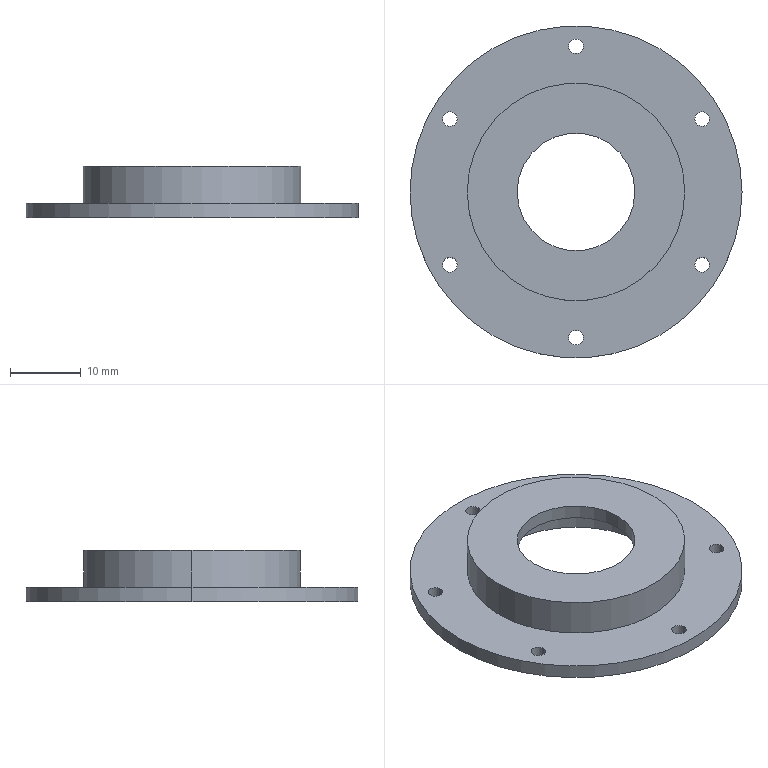Part | SolidWorks | features BaseBody 1 | 1 solid | 24 faces | box 47.022 x 47.022 x 7.237 mm | volume 3944 mm3 | cylinder 20 | plane 4 | commonest cylinder face diameters 2.063 x12 16.673 x2 26.799 x2 30.799 x2 47.022 x2
STEP:
#1=CARTESIAN_POINT('',(17.927,0.,0.));
#2=VERTEX_POINT('',#1);
#3=CARTESIAN_POINT('',(-8.872,0.,0.));
#4=VERTEX_POINT('',#3);
#5=CARTESIAN_POINT('',(4.528,0.,0.));
#6=DIRECTION('',(0.,0.,-1.));
#7=DIRECTION('',(1.,0.,0.));
#8=AXIS2_PLACEMENT_3D('',#5,#6,#7);
#9=CIRCLE('',#8,13.4);
#10=EDGE_CURVE('',#2,#4,#9,.T.);
#11=ORIENTED_EDGE('',*,*,#10,.T.);
#12=CARTESIAN_POINT('',(-8.872,0.,5.237));
#13=VERTEX_POINT('',#12);
#14=CARTESIAN_POINT('',(-8.872,0.,0.));
#15=DIRECTION('',(0.,0.,1.));
#16=VECTOR('',#15,1000.);
#17=LINE('',#14,#16);
#18=EDGE_CURVE('',#4,#13,#17,.T.);
#19=ORIENTED_EDGE('',*,*,#18,.T.);
#20=CARTESIAN_POINT('',(17.927,0.,5.237));
#21=VERTEX_POINT('',#20);
#22=CARTESIAN_POINT('',(4.528,0.,5.237));
#23=DIRECTION('',(0.,0.,-1.));
#24=DIRECTION('',(1.,0.,0.));
#25=AXIS2_PLACEMENT_3D('',#22,#23,#24);
#26=CIRCLE('',#25,13.4);
#27=EDGE_CURVE('',#21,#13,#26,.T.);
#28=ORIENTED_EDGE('',*,*,#27,.F.);
#29=CARTESIAN_POINT('',(17.927,0.,0.));
#30=DIRECTION('',(0.,0.,1.));
#31=VECTOR('',#30,1000.);
#32=LINE('',#29,#31);
#33=EDGE_CURVE('',#2,#21,#32,.T.);
#34=ORIENTED_EDGE('',*,*,#33,.F.);
#35=EDGE_LOOP('',(#11,#19,#28,#34));
#36=FACE_OUTER_BOUND('',#35,.T.);
#37=CARTESIAN_POINT('',(4.528,0.,0.));
#38=DIRECTION('',(0.,0.,1.));
#39=DIRECTION('',(1.,0.,0.));
#40=AXIS2_PLACEMENT_3D('',#37,#38,#39);
#41=CYLINDRICAL_SURFACE('',#40,13.4);
#42=ADVANCED_FACE('',(#36),#41,.F.);
#43=CARTESIAN_POINT('',(5.559,20.627,0.));
#44=VERTEX_POINT('',#43);
#45=CARTESIAN_POINT('',(3.496,20.627,0.));
#46=VERTEX_POINT('',#45);
#47=CARTESIAN_POINT('',(4.528,20.627,0.));
#48=DIRECTION('',(0.,0.,-1.));
#49=DIRECTION('',(1.,0.,0.));
#50=AXIS2_PLACEMENT_3D('',#47,#48,#49);
#51=CIRCLE('',#50,1.032);
#52=EDGE_CURVE('',#44,#46,#51,.T.);
#53=ORIENTED_EDGE('',*,*,#52,.T.);
#54=CARTESIAN_POINT('',(3.496,20.627,2.));
#55=VERTEX_POINT('',#54);
#56=CARTESIAN_POINT('',(3.496,20.627,0.));
#57=DIRECTION('',(0.,0.,1.));
#58=VECTOR('',#57,1000.);
#59=LINE('',#56,#58);
#60=EDGE_CURVE('',#46,#55,#59,.T.);
#61=ORIENTED_EDGE('',*,*,#60,.T.);
#62=CARTESIAN_POINT('',(5.559,20.627,2.));
#63=VERTEX_POINT('',#62);
#64=CARTESIAN_POINT('',(4.528,20.627,2.));
#65=DIRECTION('',(0.,0.,-1.));
#66=DIRECTION('',(1.,0.,0.));
#67=AXIS2_PLACEMENT_3D('',#64,#65,#66);
#68=CIRCLE('',#67,1.032);
#69=EDGE_CURVE('',#63,#55,#68,.T.);
#70=ORIENTED_EDGE('',*,*,#69,.F.);
#71=CARTESIAN_POINT('',(5.559,20.627,0.));
#72=DIRECTION('',(0.,0.,1.));
#73=VECTOR('',#72,1000.);
#74=LINE('',#71,#73);
#75=EDGE_CURVE('',#44,#63,#74,.T.);
#76=ORIENTED_EDGE('',*,*,#75,.F.);
#77=EDGE_LOOP('',(#53,#61,#70,#76));
#78=FACE_OUTER_BOUND('',#77,.T.);
#79=CARTESIAN_POINT('',(4.528,20.627,0.));
#80=DIRECTION('',(0.,0.,1.));
#81=DIRECTION('',(1.,0.,0.));
#82=AXIS2_PLACEMENT_3D('',#79,#80,#81);
#83=CYLINDRICAL_SURFACE('',#82,1.032);
#84=ADVANCED_FACE('',(#78),#83,.F.);
#85=CARTESIAN_POINT('',(-12.305,10.314,0.));
#86=VERTEX_POINT('',#85);
#87=CARTESIAN_POINT('',(-14.368,10.314,0.));
#88=VERTEX_POINT('',#87);
#89=CARTESIAN_POINT('',(-13.336,10.314,0.));
#90=DIRECTION('',(0.,0.,-1.));
#91=DIRECTION('',(1.,0.,0.));
#92=AXIS2_PLACEMENT_3D('',#89,#90,#91);
#93=CIRCLE('',#92,1.032);
#94=EDGE_CURVE('',#86,#88,#93,.T.);
#95=ORIENTED_EDGE('',*,*,#94,.T.);
#96=CARTESIAN_POINT('',(-14.368,10.314,2.));
#97=VERTEX_POINT('',#96);
#98=CARTESIAN_POINT('',(-14.368,10.314,0.));
#99=DIRECTION('',(0.,0.,1.));
#100=VECTOR('',#99,1000.);
#101=LINE('',#98,#100);
#102=EDGE_CURVE('',#88,#97,#101,.T.);
#103=ORIENTED_EDGE('',*,*,#102,.T.);
#104=CARTESIAN_POINT('',(-12.305,10.314,2.));
#105=VERTEX_POINT('',#104);
#106=CARTESIAN_POINT('',(-13.336,10.314,2.));
#107=DIRECTION('',(0.,0.,-1.));
#108=DIRECTION('',(1.,0.,0.));
#109=AXIS2_PLACEMENT_3D('',#106,#107,#108);
#110=CIRCLE('',#109,1.032);
#111=EDGE_CURVE('',#105,#97,#110,.T.);
#112=ORIENTED_EDGE('',*,*,#111,.F.);
#113=CARTESIAN_POINT('',(-12.305,10.314,0.));
#114=DIRECTION('',(0.,0.,1.));
#115=VECTOR('',#114,1000.);
#116=LINE('',#113,#115);
#117=EDGE_CURVE('',#86,#105,#116,.T.);
#118=ORIENTED_EDGE('',*,*,#117,.F.);
#119=EDGE_LOOP('',(#95,#103,#112,#118));
#120=FACE_OUTER_BOUND('',#119,.T.);
#121=CARTESIAN_POINT('',(-13.336,10.314,0.));
#122=DIRECTION('',(0.,0.,1.));
#123=DIRECTION('',(1.,0.,0.));
#124=AXIS2_PLACEMENT_3D('',#121,#122,#123);
#125=CYLINDRICAL_SURFACE('',#124,1.032);
#126=ADVANCED_FACE('',(#120),#125,.F.);
#127=CARTESIAN_POINT('',(-12.305,-10.314,0.));
#128=VERTEX_POINT('',#127);
#129=CARTESIAN_POINT('',(-14.368,-10.314,0.));
#130=VERTEX_POINT('',#129);
#131=CARTESIAN_POINT('',(-13.336,-10.314,0.));
#132=DIRECTION('',(0.,0.,-1.));
#133=DIRECTION('',(1.,0.,0.));
#134=AXIS2_PLACEMENT_3D('',#131,#132,#133);
#135=CIRCLE('',#134,1.032);
#136=EDGE_CURVE('',#128,#130,#135,.T.);
#137=ORIENTED_EDGE('',*,*,#136,.T.);
#138=CARTESIAN_POINT('',(-14.368,-10.314,2.));
#139=VERTEX_POINT('',#138);
#140=CARTESIAN_POINT('',(-14.368,-10.314,0.));
#141=DIRECTION('',(0.,0.,1.));
#142=VECTOR('',#141,1000.);
#143=LINE('',#140,#142);
#144=EDGE_CURVE('',#130,#139,#143,.T.);
#145=ORIENTED_EDGE('',*,*,#144,.T.);
#146=CARTESIAN_POINT('',(-12.305,-10.314,2.));
#147=VERTEX_POINT('',#146);
#148=CARTESIAN_POINT('',(-13.336,-10.314,2.));
#149=DIRECTION('',(0.,0.,-1.));
#150=DIRECTION('',(1.,0.,0.));
#151=AXIS2_PLACEMENT_3D('',#148,#149,#150);
#152=CIRCLE('',#151,1.032);
#153=EDGE_CURVE('',#147,#139,#152,.T.);
#154=ORIENTED_EDGE('',*,*,#153,.F.);
#155=CARTESIAN_POINT('',(-12.305,-10.314,0.));
#156=DIRECTION('',(0.,0.,1.));
#157=VECTOR('',#156,1000.);
#158=LINE('',#155,#157);
#159=EDGE_CURVE('',#128,#147,#158,.T.);
#160=ORIENTED_EDGE('',*,*,#159,.F.);
#161=EDGE_LOOP('',(#137,#145,#154,#160));
#162=FACE_OUTER_BOUND('',#161,.T.);
#163=CARTESIAN_POINT('',(-13.336,-10.314,0.));
#164=DIRECTION('',(0.,0.,1.));
#165=DIRECTION('',(1.,0.,0.));
#166=AXIS2_PLACEMENT_3D('',#163,#164,#165);
#167=CYLINDRICAL_SURFACE('',#166,1.032);
#168=ADVANCED_FACE('',(#162),#167,.F.);
#169=CARTESIAN_POINT('',(5.559,-20.627,0.));
#170=VERTEX_POINT('',#169);
#171=CARTESIAN_POINT('',(3.496,-20.627,0.));
#172=VERTEX_POINT('',#171);
#173=CARTESIAN_POINT('',(4.528,-20.627,0.));
#174=DIRECTION('',(0.,0.,-1.));
#175=DIRECTION('',(1.,0.,0.));
#176=AXIS2_PLACEMENT_3D('',#173,#174,#175);
#177=CIRCLE('',#176,1.032);
#178=EDGE_CURVE('',#170,#172,#177,.T.);
#179=ORIENTED_EDGE('',*,*,#178,.T.);
#180=CARTESIAN_POINT('',(3.496,-20.627,2.));
#181=VERTEX_POINT('',#180);
#182=CARTESIAN_POINT('',(3.496,-20.627,0.));
#183=DIRECTION('',(0.,0.,1.));
#184=VECTOR('',#183,1000.);
#185=LINE('',#182,#184);
#186=EDGE_CURVE('',#172,#181,#185,.T.);
#187=ORIENTED_EDGE('',*,*,#186,.T.);
#188=CARTESIAN_POINT('',(5.559,-20.627,2.));
#189=VERTEX_POINT('',#188);
#190=CARTESIAN_POINT('',(4.528,-20.627,2.));
#191=DIRECTION('',(0.,0.,-1.));
#192=DIRECTION('',(1.,0.,0.));
#193=AXIS2_PLACEMENT_3D('',#190,#191,#192);
#194=CIRCLE('',#193,1.032);
#195=EDGE_CURVE('',#189,#181,#194,.T.);
#196=ORIENTED_EDGE('',*,*,#195,.F.);
#197=CARTESIAN_POINT('',(5.559,-20.627,0.));
#198=DIRECTION('',(0.,0.,1.));
#199=VECTOR('',#198,1000.);
#200=LINE('',#197,#199);
#201=EDGE_CURVE('',#170,#189,#200,.T.);
#202=ORIENTED_EDGE('',*,*,#201,.F.);
#203=EDGE_LOOP('',(#179,#187,#196,#202));
#204=FACE_OUTER_BOUND('',#203,.T.);
#205=CARTESIAN_POINT('',(4.528,-20.627,0.));
#206=DIRECTION('',(0.,0.,1.));
#207=DIRECTION('',(1.,0.,0.));
#208=AXIS2_PLACEMENT_3D('',#205,#206,#207);
#209=CYLINDRICAL_SURFACE('',#208,1.032);
#210=ADVANCED_FACE('',(#204),#209,.F.);
#211=CARTESIAN_POINT('',(23.423,-10.314,0.));
#212=VERTEX_POINT('',#211);
#213=CARTESIAN_POINT('',(21.36,-10.314,0.));
#214=VERTEX_POINT('',#213);
#215=CARTESIAN_POINT('',(22.392,-10.314,0.));
#216=DIRECTION('',(0.,0.,-1.));
#217=DIRECTION('',(1.,0.,0.));
#218=AXIS2_PLACEMENT_3D('',#215,#216,#217);
#219=CIRCLE('',#218,1.032);
#220=EDGE_CURVE('',#212,#214,#219,.T.);
#221=ORIENTED_EDGE('',*,*,#220,.T.);
#222=CARTESIAN_POINT('',(21.36,-10.314,2.));
#223=VERTEX_POINT('',#222);
#224=CARTESIAN_POINT('',(21.36,-10.314,0.));
#225=DIRECTION('',(0.,0.,1.));
#226=VECTOR('',#225,1000.);
#227=LINE('',#224,#226);
#228=EDGE_CURVE('',#214,#223,#227,.T.);
#229=ORIENTED_EDGE('',*,*,#228,.T.);
#230=CARTESIAN_POINT('',(23.423,-10.314,2.));
#231=VERTEX_POINT('',#230);
#232=CARTESIAN_POINT('',(22.392,-10.314,2.));
#233=DIRECTION('',(0.,0.,-1.));
#234=DIRECTION('',(1.,0.,0.));
#235=AXIS2_PLACEMENT_3D('',#232,#233,#234);
#236=CIRCLE('',#235,1.032);
#237=EDGE_CURVE('',#231,#223,#236,.T.);
#238=ORIENTED_EDGE('',*,*,#237,.F.);
#239=CARTESIAN_POINT('',(23.423,-10.314,0.));
#240=DIRECTION('',(0.,0.,1.));
#241=VECTOR('',#240,1000.);
#242=LINE('',#239,#241);
#243=EDGE_CURVE('',#212,#231,#242,.T.);
#244=ORIENTED_EDGE('',*,*,#243,.F.);
#245=EDGE_LOOP('',(#221,#229,#238,#244));
#246=FACE_OUTER_BOUND('',#245,.T.);
#247=CARTESIAN_POINT('',(22.392,-10.314,0.));
#248=DIRECTION('',(0.,0.,1.));
#249=DIRECTION('',(1.,0.,0.));
#250=AXIS2_PLACEMENT_3D('',#247,#248,#249);
#251=CYLINDRICAL_SURFACE('',#250,1.032);
#252=ADVANCED_FACE('',(#246),#251,.F.);
#253=CARTESIAN_POINT('',(23.423,10.314,0.));
#254=VERTEX_POINT('',#253);
#255=CARTESIAN_POINT('',(21.36,10.314,0.));
#256=VERTEX_POINT('',#255);
#257=CARTESIAN_POINT('',(22.392,10.314,0.));
#258=DIRECTION('',(0.,0.,-1.));
#259=DIRECTION('',(1.,0.,0.));
#260=AXIS2_PLACEMENT_3D('',#257,#258,#259);
#261=CIRCLE('',#260,1.032);
#262=EDGE_CURVE('',#254,#256,#261,.T.);
#263=ORIENTED_EDGE('',*,*,#262,.T.);
#264=CARTESIAN_POINT('',(21.36,10.314,2.));
#265=VERTEX_POINT('',#264);
#266=CARTESIAN_POINT('',(21.36,10.314,0.));
#267=DIRECTION('',(0.,0.,1.));
#268=VECTOR('',#267,1000.);
#269=LINE('',#266,#268);
#270=EDGE_CURVE('',#256,#265,#269,.T.);
#271=ORIENTED_EDGE('',*,*,#270,.T.);
#272=CARTESIAN_POINT('',(23.423,10.314,2.));
#273=VERTEX_POINT('',#272);
#274=CARTESIAN_POINT('',(22.392,10.314,2.));
#275=DIRECTION('',(0.,0.,-1.));
#276=DIRECTION('',(1.,0.,0.));
#277=AXIS2_PLACEMENT_3D('',#274,#275,#276);
#278=CIRCLE('',#277,1.032);
#279=EDGE_CURVE('',#273,#265,#278,.T.);
#280=ORIENTED_EDGE('',*,*,#279,.F.);
#281=CARTESIAN_POINT('',(23.423,10.314,0.));
#282=DIRECTION('',(0.,0.,1.));
#283=VECTOR('',#282,1000.);
#284=LINE('',#281,#283);
#285=EDGE_CURVE('',#254,#273,#284,.T.);
#286=ORIENTED_EDGE('',*,*,#285,.F.);
#287=EDGE_LOOP('',(#263,#271,#280,#286));
#288=FACE_OUTER_BOUND('',#287,.T.);
#289=CARTESIAN_POINT('',(22.392,10.314,0.));
#290=DIRECTION('',(0.,0.,1.));
#291=DIRECTION('',(1.,0.,0.));
#292=AXIS2_PLACEMENT_3D('',#289,#290,#291);
#293=CYLINDRICAL_SURFACE('',#292,1.032);
#294=ADVANCED_FACE('',(#288),#293,.F.);
#295=CARTESIAN_POINT('',(28.039,0.,0.));
#296=VERTEX_POINT('',#295);
#297=CARTESIAN_POINT('',(-18.983,0.,0.));
#298=VERTEX_POINT('',#297);
#299=CARTESIAN_POINT('',(4.528,0.,0.));
#300=DIRECTION('',(0.,0.,1.));
#301=DIRECTION('',(1.,0.,0.));
#302=AXIS2_PLACEMENT_3D('',#299,#300,#301);
#303=CIRCLE('',#302,23.511);
#304=EDGE_CURVE('',#296,#298,#303,.T.);
#305=ORIENTED_EDGE('',*,*,#304,.T.);
#306=CARTESIAN_POINT('',(-18.983,0.,2.));
#307=VERTEX_POINT('',#306);
#308=CARTESIAN_POINT('',(-18.983,0.,0.));
#309=DIRECTION('',(0.,0.,1.));
#310=VECTOR('',#309,1000.);
#311=LINE('',#308,#310);
#312=EDGE_CURVE('',#298,#307,#311,.T.);
#313=ORIENTED_EDGE('',*,*,#312,.T.);
#314=CARTESIAN_POINT('',(28.039,0.,2.));
#315=VERTEX_POINT('',#314);
#316=CARTESIAN_POINT('',(4.528,0.,2.));
#317=DIRECTION('',(0.,0.,-1.));
#318=DIRECTION('',(1.,0.,0.));
#319=AXIS2_PLACEMENT_3D('',#316,#317,#318);
#320=CIRCLE('',#319,23.511);
#321=EDGE_CURVE('',#307,#315,#320,.T.);
#322=ORIENTED_EDGE('',*,*,#321,.T.);
#323=CARTESIAN_POINT('',(28.039,0.,0.));
#324=DIRECTION('',(0.,0.,1.));
#325=VECTOR('',#324,1000.);
#326=LINE('',#323,#325);
#327=EDGE_CURVE('',#296,#315,#326,.T.);
#328=ORIENTED_EDGE('',*,*,#327,.F.);
#329=EDGE_LOOP('',(#305,#313,#322,#328));
#330=FACE_OUTER_BOUND('',#329,.T.);
#331=CARTESIAN_POINT('',(4.528,0.,0.));
#332=DIRECTION('',(0.,0.,1.));
#333=DIRECTION('',(1.,0.,0.));
#334=AXIS2_PLACEMENT_3D('',#331,#332,#333);
#335=CYLINDRICAL_SURFACE('',#334,23.511);
#336=ADVANCED_FACE('',(#330),#335,.T.);
#337=CARTESIAN_POINT('',(12.864,0.,5.237));
#338=VERTEX_POINT('',#337);
#339=CARTESIAN_POINT('',(-3.809,0.,5.237));
#340=VERTEX_POINT('',#339);
#341=CARTESIAN_POINT('',(4.528,0.,5.237));
#342=DIRECTION('',(0.,0.,-1.));
#343=DIRECTION('',(1.,0.,0.));
#344=AXIS2_PLACEMENT_3D('',#341,#342,#343);
#345=CIRCLE('',#344,8.336);
#346=EDGE_CURVE('',#338,#340,#345,.T.);
#347=ORIENTED_EDGE('',*,*,#346,.T.);
#348=CARTESIAN_POINT('',(-3.809,0.,7.237));
#349=VERTEX_POINT('',#348);
#350=CARTESIAN_POINT('',(-3.809,0.,5.237));
#351=DIRECTION('',(0.,0.,1.));
#352=VECTOR('',#351,1000.);
#353=LINE('',#350,#352);
#354=EDGE_CURVE('',#340,#349,#353,.T.);
#355=ORIENTED_EDGE('',*,*,#354,.T.);
#356=CARTESIAN_POINT('',(12.864,0.,7.237));
#357=VERTEX_POINT('',#356);
#358=CARTESIAN_POINT('',(4.528,0.,7.237));
#359=DIRECTION('',(0.,0.,-1.));
#360=DIRECTION('',(1.,0.,0.));
#361=AXIS2_PLACEMENT_3D('',#358,#359,#360);
#362=CIRCLE('',#361,8.336);
#363=EDGE_CURVE('',#357,#349,#362,.T.);
#364=ORIENTED_EDGE('',*,*,#363,.F.);
#365=CARTESIAN_POINT('',(12.864,0.,5.237));
#366=DIRECTION('',(0.,0.,1.));
#367=VECTOR('',#366,1000.);
#368=LINE('',#365,#367);
#369=EDGE_CURVE('',#338,#357,#368,.T.);
#370=ORIENTED_EDGE('',*,*,#369,.F.);
#371=EDGE_LOOP('',(#347,#355,#364,#370));
#372=FACE_OUTER_BOUND('',#371,.T.);
#373=CARTESIAN_POINT('',(4.528,0.,5.237));
#374=DIRECTION('',(0.,0.,1.));
#375=DIRECTION('',(1.,0.,0.));
#376=AXIS2_PLACEMENT_3D('',#373,#374,#375);
#377=CYLINDRICAL_SURFACE('',#376,8.336);
#378=ADVANCED_FACE('',(#372),#377,.F.);
#379=CARTESIAN_POINT('',(-10.872,0.,2.));
#380=VERTEX_POINT('',#379);
#381=CARTESIAN_POINT('',(19.927,0.,2.));
#382=VERTEX_POINT('',#381);
#383=CARTESIAN_POINT('',(4.528,0.,2.));
#384=DIRECTION('',(0.,0.,-1.));
#385=DIRECTION('',(1.,0.,0.));
#386=AXIS2_PLACEMENT_3D('',#383,#384,#385);
#387=CIRCLE('',#386,15.4);
#388=EDGE_CURVE('',#380,#382,#387,.T.);
#389=ORIENTED_EDGE('',*,*,#388,.F.);
#390=CARTESIAN_POINT('',(-10.872,0.,7.237));
#391=VERTEX_POINT('',#390);
#392=CARTESIAN_POINT('',(-10.872,0.,2.));
#393=DIRECTION('',(0.,0.,1.));
#394=VECTOR('',#393,1000.);
#395=LINE('',#392,#394);
#396=EDGE_CURVE('',#380,#391,#395,.T.);
#397=ORIENTED_EDGE('',*,*,#396,.T.);
#398=CARTESIAN_POINT('',(19.927,0.,7.237));
#399=VERTEX_POINT('',#398);
#400=CARTESIAN_POINT('',(4.528,0.,7.237));
#401=DIRECTION('',(0.,0.,-1.));
#402=DIRECTION('',(1.,0.,0.));
#403=AXIS2_PLACEMENT_3D('',#400,#401,#402);
#404=CIRCLE('',#403,15.4);
#405=EDGE_CURVE('',#391,#399,#404,.T.);
#406=ORIENTED_EDGE('',*,*,#405,.T.);
#407=CARTESIAN_POINT('',(19.927,0.,2.));
#408=DIRECTION('',(0.,0.,1.));
#409=VECTOR('',#408,1000.);
#410=LINE('',#407,#409);
#411=EDGE_CURVE('',#382,#399,#410,.T.);
#412=ORIENTED_EDGE('',*,*,#411,.F.);
#413=EDGE_LOOP('',(#389,#397,#406,#412));
#414=FACE_OUTER_BOUND('',#413,.T.);
#415=CARTESIAN_POINT('',(4.528,0.,2.));
#416=DIRECTION('',(0.,0.,1.));
#417=DIRECTION('',(1.,0.,0.));
#418=AXIS2_PLACEMENT_3D('',#415,#416,#417);
#419=CYLINDRICAL_SURFACE('',#418,15.4);
#420=ADVANCED_FACE('',(#414),#419,.T.);
#421=ORIENTED_EDGE('',*,*,#10,.F.);
#422=CARTESIAN_POINT('',(4.528,0.,0.));
#423=DIRECTION('',(0.,0.,-1.));
#424=DIRECTION('',(1.,0.,0.));
#425=AXIS2_PLACEMENT_3D('',#422,#423,#424);
#426=CIRCLE('',#425,13.4);
#427=EDGE_CURVE('',#4,#2,#426,.T.);
#428=ORIENTED_EDGE('',*,*,#427,.F.);
#429=EDGE_LOOP('',(#421,#428));
#430=FACE_BOUND('',#429,.T.);
#431=ORIENTED_EDGE('',*,*,#52,.F.);
#432=CARTESIAN_POINT('',(4.528,20.627,0.));
#433=DIRECTION('',(0.,0.,-1.));
#434=DIRECTION('',(1.,0.,0.));
#435=AXIS2_PLACEMENT_3D('',#432,#433,#434);
#436=CIRCLE('',#435,1.032);
#437=EDGE_CURVE('',#46,#44,#436,.T.);
#438=ORIENTED_EDGE('',*,*,#437,.F.);
#439=EDGE_LOOP('',(#431,#438));
#440=FACE_BOUND('',#439,.T.);
#441=ORIENTED_EDGE('',*,*,#94,.F.);
#442=CARTESIAN_POINT('',(-13.336,10.314,0.));
#443=DIRECTION('',(0.,0.,-1.));
#444=DIRECTION('',(1.,0.,0.));
#445=AXIS2_PLACEMENT_3D('',#442,#443,#444);
#446=CIRCLE('',#445,1.032);
#447=EDGE_CURVE('',#88,#86,#446,.T.);
#448=ORIENTED_EDGE('',*,*,#447,.F.);
#449=EDGE_LOOP('',(#441,#448));
#450=FACE_BOUND('',#449,.T.);
#451=ORIENTED_EDGE('',*,*,#136,.F.);
#452=CARTESIAN_POINT('',(-13.336,-10.314,0.));
#453=DIRECTION('',(0.,0.,-1.));
#454=DIRECTION('',(1.,0.,0.));
#455=AXIS2_PLACEMENT_3D('',#452,#453,#454);
#456=CIRCLE('',#455,1.032);
#457=EDGE_CURVE('',#130,#128,#456,.T.);
#458=ORIENTED_EDGE('',*,*,#457,.F.);
#459=EDGE_LOOP('',(#451,#458));
#460=FACE_BOUND('',#459,.T.);
#461=ORIENTED_EDGE('',*,*,#178,.F.);
#462=CARTESIAN_POINT('',(4.528,-20.627,0.));
#463=DIRECTION('',(0.,0.,-1.));
#464=DIRECTION('',(1.,0.,0.));
#465=AXIS2_PLACEMENT_3D('',#462,#463,#464);
#466=CIRCLE('',#465,1.032);
#467=EDGE_CURVE('',#172,#170,#466,.T.);
#468=ORIENTED_EDGE('',*,*,#467,.F.);
#469=EDGE_LOOP('',(#461,#468));
#470=FACE_BOUND('',#469,.T.);
#471=ORIENTED_EDGE('',*,*,#220,.F.);
#472=CARTESIAN_POINT('',(22.392,-10.314,0.));
#473=DIRECTION('',(0.,0.,-1.));
#474=DIRECTION('',(1.,0.,0.));
#475=AXIS2_PLACEMENT_3D('',#472,#473,#474);
#476=CIRCLE('',#475,1.032);
#477=EDGE_CURVE('',#214,#212,#476,.T.);
#478=ORIENTED_EDGE('',*,*,#477,.F.);
#479=EDGE_LOOP('',(#471,#478));
#480=FACE_BOUND('',#479,.T.);
#481=ORIENTED_EDGE('',*,*,#262,.F.);
#482=CARTESIAN_POINT('',(22.392,10.314,0.));
#483=DIRECTION('',(0.,0.,-1.));
#484=DIRECTION('',(1.,0.,0.));
#485=AXIS2_PLACEMENT_3D('',#482,#483,#484);
#486=CIRCLE('',#485,1.032);
#487=EDGE_CURVE('',#256,#254,#486,.T.);
#488=ORIENTED_EDGE('',*,*,#487,.F.);
#489=EDGE_LOOP('',(#481,#488));
#490=FACE_BOUND('',#489,.T.);
#491=ORIENTED_EDGE('',*,*,#304,.F.);
#492=CARTESIAN_POINT('',(4.528,0.,0.));
#493=DIRECTION('',(0.,0.,1.));
#494=DIRECTION('',(1.,0.,0.));
#495=AXIS2_PLACEMENT_3D('',#492,#493,#494);
#496=CIRCLE('',#495,23.511);
#497=EDGE_CURVE('',#298,#296,#496,.T.);
#498=ORIENTED_EDGE('',*,*,#497,.F.);
#499=EDGE_LOOP('',(#491,#498));
#500=FACE_OUTER_BOUND('',#499,.T.);
#501=CARTESIAN_POINT('',(4.528,0.,0.));
#502=DIRECTION('',(0.,0.,1.));
#503=DIRECTION('',(1.,0.,0.));
#504=AXIS2_PLACEMENT_3D('',#501,#502,#503);
#505=PLANE('',#504);
#506=ADVANCED_FACE('',(#430,#440,#450,#460,#470,#480,#490,#500),#505,.F.);
#507=ORIENTED_EDGE('',*,*,#18,.F.);
#508=ORIENTED_EDGE('',*,*,#427,.T.);
#509=ORIENTED_EDGE('',*,*,#33,.T.);
#510=CARTESIAN_POINT('',(4.528,0.,5.237));
#511=DIRECTION('',(0.,0.,-1.));
#512=DIRECTION('',(1.,0.,0.));
#513=AXIS2_PLACEMENT_3D('',#510,#511,#512);
#514=CIRCLE('',#513,13.4);
#515=EDGE_CURVE('',#13,#21,#514,.T.);
#516=ORIENTED_EDGE('',*,*,#515,.F.);
#517=EDGE_LOOP('',(#507,#508,#509,#516));
#518=FACE_OUTER_BOUND('',#517,.T.);
#519=CARTESIAN_POINT('',(4.528,0.,0.));
#520=DIRECTION('',(0.,0.,1.));
#521=DIRECTION('',(1.,0.,0.));
#522=AXIS2_PLACEMENT_3D('',#519,#520,#521);
#523=CYLINDRICAL_SURFACE('',#522,13.4);
#524=ADVANCED_FACE('',(#518),#523,.F.);
#525=ORIENTED_EDGE('',*,*,#60,.F.);
#526=ORIENTED_EDGE('',*,*,#437,.T.);
#527=ORIENTED_EDGE('',*,*,#75,.T.);
#528=CARTESIAN_POINT('',(4.528,20.627,2.));
#529=DIRECTION('',(0.,0.,-1.));
#530=DIRECTION('',(1.,0.,0.));
#531=AXIS2_PLACEMENT_3D('',#528,#529,#530);
#532=CIRCLE('',#531,1.032);
#533=EDGE_CURVE('',#55,#63,#532,.T.);
#534=ORIENTED_EDGE('',*,*,#533,.F.);
#535=EDGE_LOOP('',(#525,#526,#527,#534));
#536=FACE_OUTER_BOUND('',#535,.T.);
#537=CARTESIAN_POINT('',(4.528,20.627,0.));
#538=DIRECTION('',(0.,0.,1.));
#539=DIRECTION('',(1.,0.,0.));
#540=AXIS2_PLACEMENT_3D('',#537,#538,#539);
#541=CYLINDRICAL_SURFACE('',#540,1.032);
#542=ADVANCED_FACE('',(#536),#541,.F.);
#543=ORIENTED_EDGE('',*,*,#102,.F.);
#544=ORIENTED_EDGE('',*,*,#447,.T.);
#545=ORIENTED_EDGE('',*,*,#117,.T.);
#546=CARTESIAN_POINT('',(-13.336,10.314,2.));
#547=DIRECTION('',(0.,0.,-1.));
#548=DIRECTION('',(1.,0.,0.));
#549=AXIS2_PLACEMENT_3D('',#546,#547,#548);
#550=CIRCLE('',#549,1.032);
#551=EDGE_CURVE('',#97,#105,#550,.T.);
#552=ORIENTED_EDGE('',*,*,#551,.F.);
#553=EDGE_LOOP('',(#543,#544,#545,#552));
#554=FACE_OUTER_BOUND('',#553,.T.);
#555=CARTESIAN_POINT('',(-13.336,10.314,0.));
#556=DIRECTION('',(0.,0.,1.));
#557=DIRECTION('',(1.,0.,0.));
#558=AXIS2_PLACEMENT_3D('',#555,#556,#557);
#559=CYLINDRICAL_SURFACE('',#558,1.032);
#560=ADVANCED_FACE('',(#554),#559,.F.);
#561=ORIENTED_EDGE('',*,*,#144,.F.);
#562=ORIENTED_EDGE('',*,*,#457,.T.);
#563=ORIENTED_EDGE('',*,*,#159,.T.);
#564=CARTESIAN_POINT('',(-13.336,-10.314,2.));
#565=DIRECTION('',(0.,0.,-1.));
#566=DIRECTION('',(1.,0.,0.));
#567=AXIS2_PLACEMENT_3D('',#564,#565,#566);
#568=CIRCLE('',#567,1.032);
#569=EDGE_CURVE('',#139,#147,#568,.T.);
#570=ORIENTED_EDGE('',*,*,#569,.F.);
#571=EDGE_LOOP('',(#561,#562,#563,#570));
#572=FACE_OUTER_BOUND('',#571,.T.);
#573=CARTESIAN_POINT('',(-13.336,-10.314,0.));
#574=DIRECTION('',(0.,0.,1.));
#575=DIRECTION('',(1.,0.,0.));
#576=AXIS2_PLACEMENT_3D('',#573,#574,#575);
#577=CYLINDRICAL_SURFACE('',#576,1.032);
#578=ADVANCED_FACE('',(#572),#577,.F.);
#579=ORIENTED_EDGE('',*,*,#186,.F.);
#580=ORIENTED_EDGE('',*,*,#467,.T.);
#581=ORIENTED_EDGE('',*,*,#201,.T.);
#582=CARTESIAN_POINT('',(4.528,-20.627,2.));
#583=DIRECTION('',(0.,0.,-1.));
#584=DIRECTION('',(1.,0.,0.));
#585=AXIS2_PLACEMENT_3D('',#582,#583,#584);
#586=CIRCLE('',#585,1.032);
#587=EDGE_CURVE('',#181,#189,#586,.T.);
#588=ORIENTED_EDGE('',*,*,#587,.F.);
#589=EDGE_LOOP('',(#579,#580,#581,#588));
#590=FACE_OUTER_BOUND('',#589,.T.);
#591=CARTESIAN_POINT('',(4.528,-20.627,0.));
#592=DIRECTION('',(0.,0.,1.));
#593=DIRECTION('',(1.,0.,0.));
#594=AXIS2_PLACEMENT_3D('',#591,#592,#593);
#595=CYLINDRICAL_SURFACE('',#594,1.032);
#596=ADVANCED_FACE('',(#590),#595,.F.);
#597=ORIENTED_EDGE('',*,*,#228,.F.);
#598=ORIENTED_EDGE('',*,*,#477,.T.);
#599=ORIENTED_EDGE('',*,*,#243,.T.);
#600=CARTESIAN_POINT('',(22.392,-10.314,2.));
#601=DIRECTION('',(0.,0.,-1.));
#602=DIRECTION('',(1.,0.,0.));
#603=AXIS2_PLACEMENT_3D('',#600,#601,#602);
#604=CIRCLE('',#603,1.032);
#605=EDGE_CURVE('',#223,#231,#604,.T.);
#606=ORIENTED_EDGE('',*,*,#605,.F.);
#607=EDGE_LOOP('',(#597,#598,#599,#606));
#608=FACE_OUTER_BOUND('',#607,.T.);
#609=CARTESIAN_POINT('',(22.392,-10.314,0.));
#610=DIRECTION('',(0.,0.,1.));
#611=DIRECTION('',(1.,0.,0.));
#612=AXIS2_PLACEMENT_3D('',#609,#610,#611);
#613=CYLINDRICAL_SURFACE('',#612,1.032);
#614=ADVANCED_FACE('',(#608),#613,.F.);
#615=ORIENTED_EDGE('',*,*,#270,.F.);
#616=ORIENTED_EDGE('',*,*,#487,.T.);
#617=ORIENTED_EDGE('',*,*,#285,.T.);
#618=CARTESIAN_POINT('',(22.392,10.314,2.));
#619=DIRECTION('',(0.,0.,-1.));
#620=DIRECTION('',(1.,0.,0.));
#621=AXIS2_PLACEMENT_3D('',#618,#619,#620);
#622=CIRCLE('',#621,1.032);
#623=EDGE_CURVE('',#265,#273,#622,.T.);
#624=ORIENTED_EDGE('',*,*,#623,.F.);
#625=EDGE_LOOP('',(#615,#616,#617,#624));
#626=FACE_OUTER_BOUND('',#625,.T.);
#627=CARTESIAN_POINT('',(22.392,10.314,0.));
#628=DIRECTION('',(0.,0.,1.));
#629=DIRECTION('',(1.,0.,0.));
#630=AXIS2_PLACEMENT_3D('',#627,#628,#629);
#631=CYLINDRICAL_SURFACE('',#630,1.032);
#632=ADVANCED_FACE('',(#626),#631,.F.);
#633=ORIENTED_EDGE('',*,*,#312,.F.);
#634=ORIENTED_EDGE('',*,*,#497,.T.);
#635=ORIENTED_EDGE('',*,*,#327,.T.);
#636=CARTESIAN_POINT('',(4.528,0.,2.));
#637=DIRECTION('',(0.,0.,-1.));
#638=DIRECTION('',(1.,0.,0.));
#639=AXIS2_PLACEMENT_3D('',#636,#637,#638);
#640=CIRCLE('',#639,23.511);
#641=EDGE_CURVE('',#315,#307,#640,.T.);
#642=ORIENTED_EDGE('',*,*,#641,.T.);
#643=EDGE_LOOP('',(#633,#634,#635,#642));
#644=FACE_OUTER_BOUND('',#643,.T.);
#645=CARTESIAN_POINT('',(4.528,0.,0.));
#646=DIRECTION('',(0.,0.,1.));
#647=DIRECTION('',(1.,0.,0.));
#648=AXIS2_PLACEMENT_3D('',#645,#646,#647);
#649=CYLINDRICAL_SURFACE('',#648,23.511);
#650=ADVANCED_FACE('',(#644),#649,.T.);
#651=ORIENTED_EDGE('',*,*,#346,.F.);
#652=CARTESIAN_POINT('',(4.528,0.,5.237));
#653=DIRECTION('',(0.,0.,-1.));
#654=DIRECTION('',(1.,0.,0.));
#655=AXIS2_PLACEMENT_3D('',#652,#653,#654);
#656=CIRCLE('',#655,8.336);
#657=EDGE_CURVE('',#340,#338,#656,.T.);
#658=ORIENTED_EDGE('',*,*,#657,.F.);
#659=EDGE_LOOP('',(#651,#658));
#660=FACE_BOUND('',#659,.T.);
#661=ORIENTED_EDGE('',*,*,#27,.T.);
#662=ORIENTED_EDGE('',*,*,#515,.T.);
#663=EDGE_LOOP('',(#661,#662));
#664=FACE_OUTER_BOUND('',#663,.T.);
#665=CARTESIAN_POINT('',(4.528,0.,5.237));
#666=DIRECTION('',(0.,0.,1.));
#667=DIRECTION('',(1.,0.,0.));
#668=AXIS2_PLACEMENT_3D('',#665,#666,#667);
#669=PLANE('',#668);
#670=ADVANCED_FACE('',(#660,#664),#669,.F.);
#671=ORIENTED_EDGE('',*,*,#69,.T.);
#672=ORIENTED_EDGE('',*,*,#533,.T.);
#673=EDGE_LOOP('',(#671,#672));
#674=FACE_BOUND('',#673,.T.);
#675=ORIENTED_EDGE('',*,*,#111,.T.);
#676=ORIENTED_EDGE('',*,*,#551,.T.);
#677=EDGE_LOOP('',(#675,#676));
#678=FACE_BOUND('',#677,.T.);
#679=ORIENTED_EDGE('',*,*,#153,.T.);
#680=ORIENTED_EDGE('',*,*,#569,.T.);
#681=EDGE_LOOP('',(#679,#680));
#682=FACE_BOUND('',#681,.T.);
#683=ORIENTED_EDGE('',*,*,#195,.T.);
#684=ORIENTED_EDGE('',*,*,#587,.T.);
#685=EDGE_LOOP('',(#683,#684));
#686=FACE_BOUND('',#685,.T.);
#687=ORIENTED_EDGE('',*,*,#237,.T.);
#688=ORIENTED_EDGE('',*,*,#605,.T.);
#689=EDGE_LOOP('',(#687,#688));
#690=FACE_BOUND('',#689,.T.);
#691=ORIENTED_EDGE('',*,*,#279,.T.);
#692=ORIENTED_EDGE('',*,*,#623,.T.);
#693=EDGE_LOOP('',(#691,#692));
#694=FACE_BOUND('',#693,.T.);
#695=CARTESIAN_POINT('',(4.528,0.,2.));
#696=DIRECTION('',(0.,0.,-1.));
#697=DIRECTION('',(1.,0.,0.));
#698=AXIS2_PLACEMENT_3D('',#695,#696,#697);
#699=CIRCLE('',#698,15.4);
#700=EDGE_CURVE('',#382,#380,#699,.T.);
#701=ORIENTED_EDGE('',*,*,#700,.T.);
#702=ORIENTED_EDGE('',*,*,#388,.T.);
#703=EDGE_LOOP('',(#701,#702));
#704=FACE_BOUND('',#703,.T.);
#705=ORIENTED_EDGE('',*,*,#641,.F.);
#706=ORIENTED_EDGE('',*,*,#321,.F.);
#707=EDGE_LOOP('',(#705,#706));
#708=FACE_OUTER_BOUND('',#707,.T.);
#709=CARTESIAN_POINT('',(4.528,0.,2.));
#710=DIRECTION('',(0.,0.,1.));
#711=DIRECTION('',(1.,0.,0.));
#712=AXIS2_PLACEMENT_3D('',#709,#710,#711);
#713=PLANE('',#712);
#714=ADVANCED_FACE('',(#674,#678,#682,#686,#690,#694,#704,#708),#713,.T.);
#715=ORIENTED_EDGE('',*,*,#354,.F.);
#716=ORIENTED_EDGE('',*,*,#657,.T.);
#717=ORIENTED_EDGE('',*,*,#369,.T.);
#718=CARTESIAN_POINT('',(4.528,0.,7.237));
#719=DIRECTION('',(0.,0.,-1.));
#720=DIRECTION('',(1.,0.,0.));
#721=AXIS2_PLACEMENT_3D('',#718,#719,#720);
#722=CIRCLE('',#721,8.336);
#723=EDGE_CURVE('',#349,#357,#722,.T.);
#724=ORIENTED_EDGE('',*,*,#723,.F.);
#725=EDGE_LOOP('',(#715,#716,#717,#724));
#726=FACE_OUTER_BOUND('',#725,.T.);
#727=CARTESIAN_POINT('',(4.528,0.,5.237));
#728=DIRECTION('',(0.,0.,1.));
#729=DIRECTION('',(1.,0.,0.));
#730=AXIS2_PLACEMENT_3D('',#727,#728,#729);
#731=CYLINDRICAL_SURFACE('',#730,8.336);
#732=ADVANCED_FACE('',(#726),#731,.F.);
#733=ORIENTED_EDGE('',*,*,#396,.F.);
#734=ORIENTED_EDGE('',*,*,#700,.F.);
#735=ORIENTED_EDGE('',*,*,#411,.T.);
#736=CARTESIAN_POINT('',(4.528,0.,7.237));
#737=DIRECTION('',(0.,0.,-1.));
#738=DIRECTION('',(1.,0.,0.));
#739=AXIS2_PLACEMENT_3D('',#736,#737,#738);
#740=CIRCLE('',#739,15.4);
#741=EDGE_CURVE('',#399,#391,#740,.T.);
#742=ORIENTED_EDGE('',*,*,#741,.T.);
#743=EDGE_LOOP('',(#733,#734,#735,#742));
#744=FACE_OUTER_BOUND('',#743,.T.);
#745=CARTESIAN_POINT('',(4.528,0.,2.));
#746=DIRECTION('',(0.,0.,1.));
#747=DIRECTION('',(1.,0.,0.));
#748=AXIS2_PLACEMENT_3D('',#745,#746,#747);
#749=CYLINDRICAL_SURFACE('',#748,15.4);
#750=ADVANCED_FACE('',(#744),#749,.T.);
#751=ORIENTED_EDGE('',*,*,#363,.T.);
#752=ORIENTED_EDGE('',*,*,#723,.T.);
#753=EDGE_LOOP('',(#751,#752));
#754=FACE_BOUND('',#753,.T.);
#755=ORIENTED_EDGE('',*,*,#741,.F.);
#756=ORIENTED_EDGE('',*,*,#405,.F.);
#757=EDGE_LOOP('',(#755,#756));
#758=FACE_OUTER_BOUND('',#757,.T.);
#759=CARTESIAN_POINT('',(4.528,0.,7.237));
#760=DIRECTION('',(0.,0.,1.));
#761=DIRECTION('',(1.,0.,0.));
#762=AXIS2_PLACEMENT_3D('',#759,#760,#761);
#763=PLANE('',#762);
#764=ADVANCED_FACE('',(#754,#758),#763,.T.);
#765=CLOSED_SHELL('',(#42,#84,#126,#168,#210,#252,#294,#336,#378,#420,#506,#524,#542,#560,#578,#596,#614,#632,#650,#670,#714,#732,#750,#764));
#766=MANIFOLD_SOLID_BREP('',#765);
#767=CARTESIAN_POINT('',(0.,0.,0.));
#768=DIRECTION('',(0.,0.,1.));
#769=DIRECTION('',(1.,0.,0.));
#770=AXIS2_PLACEMENT_3D('',#767,#768,#769);
#771=(LENGTH_UNIT()NAMED_UNIT(*)SI_UNIT(.MILLI.,.METRE.));
#772=UNCERTAINTY_MEASURE_WITH_UNIT(LENGTH_MEASURE(0.00001),#771,'','');
#773=(NAMED_UNIT(*)PLANE_ANGLE_UNIT()SI_UNIT($,.RADIAN.));
#774=(NAMED_UNIT(*)SI_UNIT($,.STERADIAN.)SOLID_ANGLE_UNIT());
#775=(GEOMETRIC_REPRESENTATION_CONTEXT(3)GLOBAL_UNCERTAINTY_ASSIGNED_CONTEXT((#772))GLOBAL_UNIT_ASSIGNED_CONTEXT((#771,#773,#774))REPRESENTATION_CONTEXT('',''));
#776=ADVANCED_BREP_SHAPE_REPRESENTATION('',(#766,#770),#775);